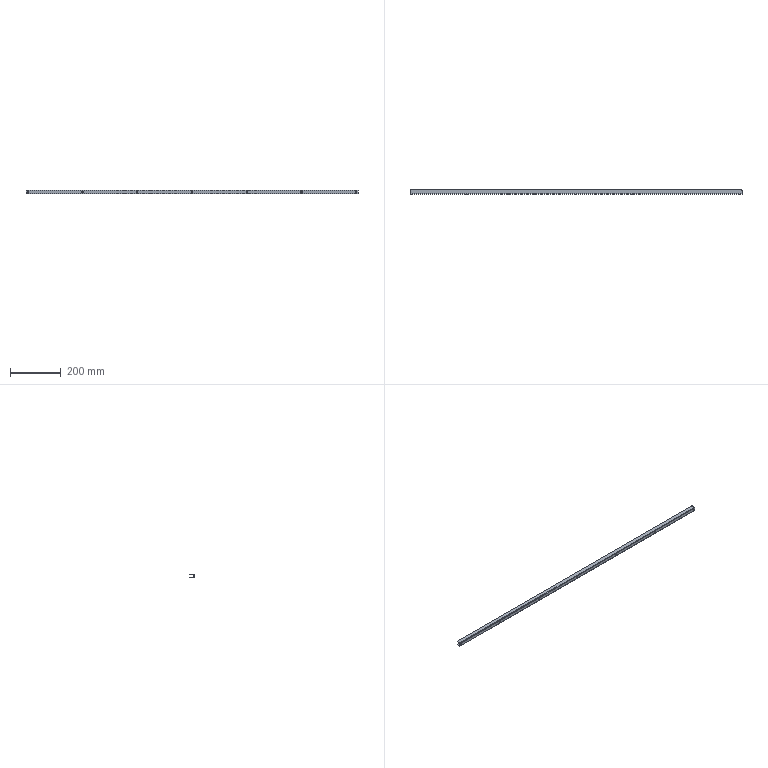Part | NX | features BREP 1 | 1 solid | 61 faces | box 1304 x 17 x 15 mm | volume 59344 mm3 | plane 32 | cylinder 29 | commonest cylinder face diameters 4.8 x21 4 x6 2 x2